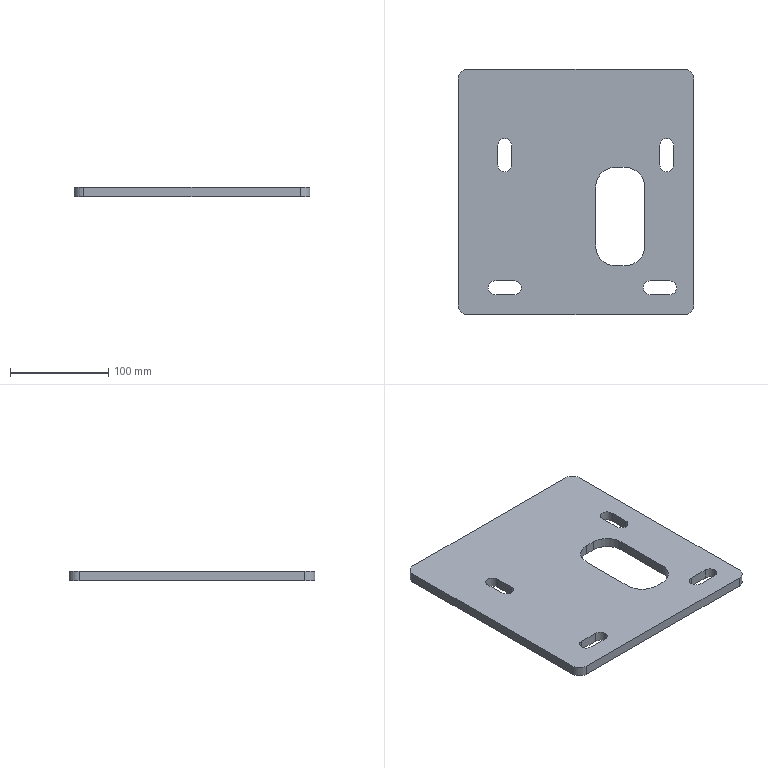Part | STEP file | IN-01-01-01-08 | 1 solid | 36 faces | box 240 x 250 x 10 mm | volume 535218 mm3 | cylinder 18 | plane 18 | commonest cylinder face diameters 14 x10 20 x4 40 x4